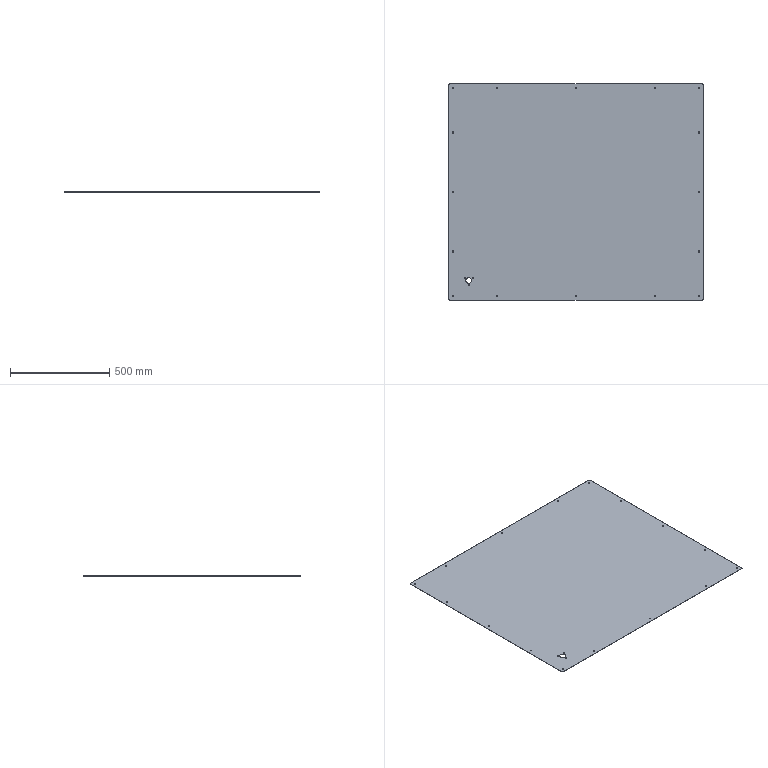Part | SolidWorks | features HoleWzd 2, Cut 1, Extrusion 1, Fillet 1 | 1 solid | 50 faces | box 1283 x 1093 x 1.5 mm | volume 2101440 mm3 | cylinder 44 | plane 6 | commonest cylinder face diameters 6.5 x38 10 x4 30 x2